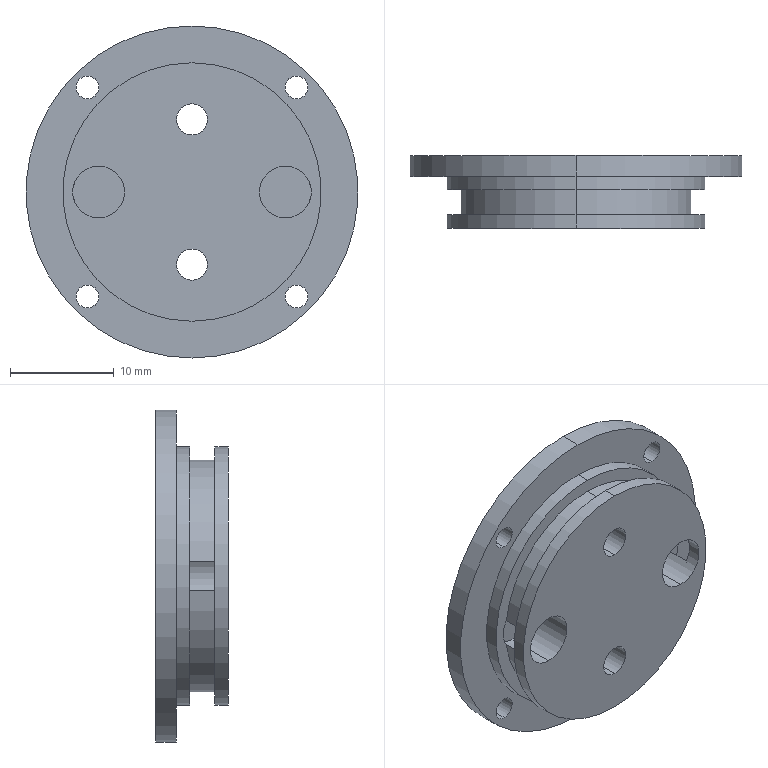Part | SolidWorks | features ICE 2, HoleWzd 1, Revolution 1 | 1 solid | 32 faces | box 32 x 7 x 32 mm | volume 3489 mm3 | cylinder 25 | plane 7 | commonest cylinder face diameters 2.2 x8 3 x4 5 x4 24.9 x4 22.309 x3 32 x2
STEP:
#1=CARTESIAN_POINT('',(0.,7.,-5.5));
#2=VERTEX_POINT('',#1);
#3=CARTESIAN_POINT('',(0.,7.,-8.5));
#4=VERTEX_POINT('',#3);
#5=CARTESIAN_POINT('',(0.,7.,-7.));
#6=DIRECTION('',(0.,-1.,0.));
#7=DIRECTION('',(0.,0.,-1.));
#8=AXIS2_PLACEMENT_3D('',#5,#6,#7);
#9=CIRCLE('',#8,1.5);
#10=EDGE_CURVE('',#2,#4,#9,.T.);
#11=ORIENTED_EDGE('',*,*,#10,.F.);
#12=CARTESIAN_POINT('',(0.,0.,-5.5));
#13=VERTEX_POINT('',#12);
#14=CARTESIAN_POINT('',(0.,5.,-5.5));
#15=DIRECTION('',(0.,-1.,0.));
#16=VECTOR('',#15,1000.);
#17=LINE('',#14,#16);
#18=EDGE_CURVE('',#2,#13,#17,.T.);
#19=ORIENTED_EDGE('',*,*,#18,.T.);
#20=CARTESIAN_POINT('',(0.,0.,-8.5));
#21=VERTEX_POINT('',#20);
#22=CARTESIAN_POINT('',(0.,0.,-7.));
#23=DIRECTION('',(0.,-1.,0.));
#24=DIRECTION('',(0.,0.,-1.));
#25=AXIS2_PLACEMENT_3D('',#22,#23,#24);
#26=CIRCLE('',#25,1.5);
#27=EDGE_CURVE('',#13,#21,#26,.T.);
#28=ORIENTED_EDGE('',*,*,#27,.T.);
#29=CARTESIAN_POINT('',(0.,5.,-8.5));
#30=DIRECTION('',(0.,-1.,0.));
#31=VECTOR('',#30,1000.);
#32=LINE('',#29,#31);
#33=EDGE_CURVE('',#4,#21,#32,.T.);
#34=ORIENTED_EDGE('',*,*,#33,.F.);
#35=EDGE_LOOP('',(#11,#19,#28,#34));
#36=FACE_OUTER_BOUND('',#35,.T.);
#37=CARTESIAN_POINT('',(0.,5.,-7.));
#38=DIRECTION('',(0.,-1.,0.));
#39=DIRECTION('',(0.,0.,-1.));
#40=AXIS2_PLACEMENT_3D('',#37,#38,#39);
#41=CYLINDRICAL_SURFACE('',#40,1.5);
#42=ADVANCED_FACE('',(#36),#41,.F.);
#43=CARTESIAN_POINT('',(0.,7.,8.5));
#44=VERTEX_POINT('',#43);
#45=CARTESIAN_POINT('',(0.,7.,5.5));
#46=VERTEX_POINT('',#45);
#47=CARTESIAN_POINT('',(0.,7.,7.));
#48=DIRECTION('',(0.,-1.,0.));
#49=DIRECTION('',(0.,0.,-1.));
#50=AXIS2_PLACEMENT_3D('',#47,#48,#49);
#51=CIRCLE('',#50,1.5);
#52=EDGE_CURVE('',#44,#46,#51,.T.);
#53=ORIENTED_EDGE('',*,*,#52,.F.);
#54=CARTESIAN_POINT('',(0.,0.,8.5));
#55=VERTEX_POINT('',#54);
#56=CARTESIAN_POINT('',(0.,5.,8.5));
#57=DIRECTION('',(0.,-1.,0.));
#58=VECTOR('',#57,1000.);
#59=LINE('',#56,#58);
#60=EDGE_CURVE('',#44,#55,#59,.T.);
#61=ORIENTED_EDGE('',*,*,#60,.T.);
#62=CARTESIAN_POINT('',(0.,0.,5.5));
#63=VERTEX_POINT('',#62);
#64=CARTESIAN_POINT('',(0.,0.,7.));
#65=DIRECTION('',(0.,-1.,0.));
#66=DIRECTION('',(0.,0.,-1.));
#67=AXIS2_PLACEMENT_3D('',#64,#65,#66);
#68=CIRCLE('',#67,1.5);
#69=EDGE_CURVE('',#55,#63,#68,.T.);
#70=ORIENTED_EDGE('',*,*,#69,.T.);
#71=CARTESIAN_POINT('',(0.,5.,5.5));
#72=DIRECTION('',(0.,-1.,0.));
#73=VECTOR('',#72,1000.);
#74=LINE('',#71,#73);
#75=EDGE_CURVE('',#46,#63,#74,.T.);
#76=ORIENTED_EDGE('',*,*,#75,.F.);
#77=EDGE_LOOP('',(#53,#61,#70,#76));
#78=FACE_OUTER_BOUND('',#77,.T.);
#79=CARTESIAN_POINT('',(0.,5.,7.));
#80=DIRECTION('',(0.,-1.,0.));
#81=DIRECTION('',(0.,0.,-1.));
#82=AXIS2_PLACEMENT_3D('',#79,#80,#81);
#83=CYLINDRICAL_SURFACE('',#82,1.5);
#84=ADVANCED_FACE('',(#78),#83,.F.);
#85=CARTESIAN_POINT('',(-11.065,3.708,1.409));
#86=VERTEX_POINT('',#85);
#87=CARTESIAN_POINT('',(-11.065,1.295,1.409));
#88=VERTEX_POINT('',#87);
#89=CARTESIAN_POINT('',(-11.065,2.5,1.409));
#90=DIRECTION('',(0.,-1.,0.));
#91=VECTOR('',#90,1000.);
#92=LINE('',#89,#91);
#93=EDGE_CURVE('',#86,#88,#92,.T.);
#94=ORIENTED_EDGE('',*,*,#93,.F.);
#95=CARTESIAN_POINT('',(-11.065,3.708,-1.409));
#96=VERTEX_POINT('',#95);
#97=CARTESIAN_POINT('',(-9.,3.708,0.));
#98=DIRECTION('',(0.,1.,0.));
#99=DIRECTION('',(0.,0.,1.));
#100=AXIS2_PLACEMENT_3D('',#97,#98,#99);
#101=CIRCLE('',#100,2.5);
#102=EDGE_CURVE('',#96,#86,#101,.T.);
#103=ORIENTED_EDGE('',*,*,#102,.F.);
#104=CARTESIAN_POINT('',(-11.065,1.295,-1.409));
#105=VERTEX_POINT('',#104);
#106=CARTESIAN_POINT('',(-11.065,2.5,-1.409));
#107=DIRECTION('',(0.,1.,0.));
#108=VECTOR('',#107,1000.);
#109=LINE('',#106,#108);
#110=EDGE_CURVE('',#105,#96,#109,.T.);
#111=ORIENTED_EDGE('',*,*,#110,.F.);
#112=CARTESIAN_POINT('',(-9.,1.295,0.));
#113=DIRECTION('',(0.,-1.,0.));
#114=DIRECTION('',(0.,0.,-1.));
#115=AXIS2_PLACEMENT_3D('',#112,#113,#114);
#116=CIRCLE('',#115,2.5);
#117=EDGE_CURVE('',#88,#105,#116,.T.);
#118=ORIENTED_EDGE('',*,*,#117,.F.);
#119=EDGE_LOOP('',(#94,#103,#111,#118));
#120=FACE_BOUND('',#119,.T.);
#121=CARTESIAN_POINT('',(-9.,5.,2.5));
#122=VERTEX_POINT('',#121);
#123=CARTESIAN_POINT('',(-9.,5.,-2.5));
#124=VERTEX_POINT('',#123);
#125=CARTESIAN_POINT('',(-9.,5.,0.));
#126=DIRECTION('',(0.,-1.,0.));
#127=DIRECTION('',(0.,0.,-1.));
#128=AXIS2_PLACEMENT_3D('',#125,#126,#127);
#129=CIRCLE('',#128,2.5);
#130=EDGE_CURVE('',#122,#124,#129,.T.);
#131=ORIENTED_EDGE('',*,*,#130,.F.);
#132=CARTESIAN_POINT('',(-9.,0.,2.5));
#133=VERTEX_POINT('',#132);
#134=CARTESIAN_POINT('',(-9.,5.,2.5));
#135=DIRECTION('',(0.,-1.,0.));
#136=VECTOR('',#135,1000.);
#137=LINE('',#134,#136);
#138=EDGE_CURVE('',#122,#133,#137,.T.);
#139=ORIENTED_EDGE('',*,*,#138,.T.);
#140=CARTESIAN_POINT('',(-9.,0.,-2.5));
#141=VERTEX_POINT('',#140);
#142=CARTESIAN_POINT('',(-9.,0.,0.));
#143=DIRECTION('',(0.,-1.,0.));
#144=DIRECTION('',(0.,0.,-1.));
#145=AXIS2_PLACEMENT_3D('',#142,#143,#144);
#146=CIRCLE('',#145,2.5);
#147=EDGE_CURVE('',#133,#141,#146,.T.);
#148=ORIENTED_EDGE('',*,*,#147,.T.);
#149=CARTESIAN_POINT('',(-9.,5.,-2.5));
#150=DIRECTION('',(0.,-1.,0.));
#151=VECTOR('',#150,1000.);
#152=LINE('',#149,#151);
#153=EDGE_CURVE('',#124,#141,#152,.T.);
#154=ORIENTED_EDGE('',*,*,#153,.F.);
#155=EDGE_LOOP('',(#131,#139,#148,#154));
#156=FACE_OUTER_BOUND('',#155,.T.);
#157=CARTESIAN_POINT('',(-9.,5.,0.));
#158=DIRECTION('',(0.,-1.,0.));
#159=DIRECTION('',(0.,0.,-1.));
#160=AXIS2_PLACEMENT_3D('',#157,#158,#159);
#161=CYLINDRICAL_SURFACE('',#160,2.5);
#162=ADVANCED_FACE('',(#120,#156),#161,.F.);
#163=CARTESIAN_POINT('',(9.,5.,2.5));
#164=VERTEX_POINT('',#163);
#165=CARTESIAN_POINT('',(9.,5.,-2.5));
#166=VERTEX_POINT('',#165);
#167=CARTESIAN_POINT('',(9.,5.,0.));
#168=DIRECTION('',(0.,-1.,0.));
#169=DIRECTION('',(0.,0.,-1.));
#170=AXIS2_PLACEMENT_3D('',#167,#168,#169);
#171=CIRCLE('',#170,2.5);
#172=EDGE_CURVE('',#164,#166,#171,.T.);
#173=ORIENTED_EDGE('',*,*,#172,.F.);
#174=CARTESIAN_POINT('',(9.,0.,2.5));
#175=VERTEX_POINT('',#174);
#176=CARTESIAN_POINT('',(9.,5.,2.5));
#177=DIRECTION('',(0.,-1.,0.));
#178=VECTOR('',#177,1000.);
#179=LINE('',#176,#178);
#180=EDGE_CURVE('',#164,#175,#179,.T.);
#181=ORIENTED_EDGE('',*,*,#180,.T.);
#182=CARTESIAN_POINT('',(9.,0.,-2.5));
#183=VERTEX_POINT('',#182);
#184=CARTESIAN_POINT('',(9.,0.,0.));
#185=DIRECTION('',(0.,-1.,0.));
#186=DIRECTION('',(0.,0.,-1.));
#187=AXIS2_PLACEMENT_3D('',#184,#185,#186);
#188=CIRCLE('',#187,2.5);
#189=EDGE_CURVE('',#175,#183,#188,.T.);
#190=ORIENTED_EDGE('',*,*,#189,.T.);
#191=CARTESIAN_POINT('',(9.,5.,-2.5));
#192=DIRECTION('',(0.,-1.,0.));
#193=VECTOR('',#192,1000.);
#194=LINE('',#191,#193);
#195=EDGE_CURVE('',#166,#183,#194,.T.);
#196=ORIENTED_EDGE('',*,*,#195,.F.);
#197=EDGE_LOOP('',(#173,#181,#190,#196));
#198=FACE_OUTER_BOUND('',#197,.T.);
#199=CARTESIAN_POINT('',(9.,5.,0.));
#200=DIRECTION('',(0.,-1.,0.));
#201=DIRECTION('',(0.,0.,-1.));
#202=AXIS2_PLACEMENT_3D('',#199,#200,#201);
#203=CYLINDRICAL_SURFACE('',#202,2.5);
#204=ADVANCED_FACE('',(#198),#203,.F.);
#205=CARTESIAN_POINT('',(-10.076,5.,-11.176));
#206=VERTEX_POINT('',#205);
#207=CARTESIAN_POINT('',(-10.076,5.,-8.976));
#208=VERTEX_POINT('',#207);
#209=CARTESIAN_POINT('',(-10.076,5.,-10.076));
#210=DIRECTION('',(0.,1.,0.));
#211=DIRECTION('',(0.,0.,1.));
#212=AXIS2_PLACEMENT_3D('',#209,#210,#211);
#213=CIRCLE('',#212,1.1);
#214=EDGE_CURVE('',#206,#208,#213,.T.);
#215=ORIENTED_EDGE('',*,*,#214,.F.);
#216=CARTESIAN_POINT('',(-10.076,7.,-11.176));
#217=VERTEX_POINT('',#216);
#218=CARTESIAN_POINT('',(-10.076,7.,-11.176));
#219=DIRECTION('',(0.,1.,0.));
#220=VECTOR('',#219,1000.);
#221=LINE('',#218,#220);
#222=EDGE_CURVE('',#206,#217,#221,.T.);
#223=ORIENTED_EDGE('',*,*,#222,.T.);
#224=CARTESIAN_POINT('',(-10.076,7.,-8.976));
#225=VERTEX_POINT('',#224);
#226=CARTESIAN_POINT('',(-10.076,7.,-10.076));
#227=DIRECTION('',(0.,1.,0.));
#228=DIRECTION('',(0.,0.,1.));
#229=AXIS2_PLACEMENT_3D('',#226,#227,#228);
#230=CIRCLE('',#229,1.1);
#231=EDGE_CURVE('',#217,#225,#230,.T.);
#232=ORIENTED_EDGE('',*,*,#231,.T.);
#233=CARTESIAN_POINT('',(-10.076,7.,-8.976));
#234=DIRECTION('',(0.,1.,0.));
#235=VECTOR('',#234,1000.);
#236=LINE('',#233,#235);
#237=EDGE_CURVE('',#208,#225,#236,.T.);
#238=ORIENTED_EDGE('',*,*,#237,.F.);
#239=EDGE_LOOP('',(#215,#223,#232,#238));
#240=FACE_OUTER_BOUND('',#239,.T.);
#241=CARTESIAN_POINT('',(-10.076,7.,-10.076));
#242=DIRECTION('',(0.,1.,0.));
#243=DIRECTION('',(0.,0.,1.));
#244=AXIS2_PLACEMENT_3D('',#241,#242,#243);
#245=CYLINDRICAL_SURFACE('',#244,1.1);
#246=ADVANCED_FACE('',(#240),#245,.F.);
#247=CARTESIAN_POINT('',(10.076,5.,-11.176));
#248=VERTEX_POINT('',#247);
#249=CARTESIAN_POINT('',(10.076,5.,-8.976));
#250=VERTEX_POINT('',#249);
#251=CARTESIAN_POINT('',(10.076,5.,-10.076));
#252=DIRECTION('',(0.,1.,0.));
#253=DIRECTION('',(0.,0.,1.));
#254=AXIS2_PLACEMENT_3D('',#251,#252,#253);
#255=CIRCLE('',#254,1.1);
#256=EDGE_CURVE('',#248,#250,#255,.T.);
#257=ORIENTED_EDGE('',*,*,#256,.F.);
#258=CARTESIAN_POINT('',(10.076,7.,-11.176));
#259=VERTEX_POINT('',#258);
#260=CARTESIAN_POINT('',(10.076,7.,-11.176));
#261=DIRECTION('',(0.,1.,0.));
#262=VECTOR('',#261,1000.);
#263=LINE('',#260,#262);
#264=EDGE_CURVE('',#248,#259,#263,.T.);
#265=ORIENTED_EDGE('',*,*,#264,.T.);
#266=CARTESIAN_POINT('',(10.076,7.,-8.976));
#267=VERTEX_POINT('',#266);
#268=CARTESIAN_POINT('',(10.076,7.,-10.076));
#269=DIRECTION('',(0.,1.,0.));
#270=DIRECTION('',(0.,0.,1.));
#271=AXIS2_PLACEMENT_3D('',#268,#269,#270);
#272=CIRCLE('',#271,1.1);
#273=EDGE_CURVE('',#259,#267,#272,.T.);
#274=ORIENTED_EDGE('',*,*,#273,.T.);
#275=CARTESIAN_POINT('',(10.076,7.,-8.976));
#276=DIRECTION('',(0.,1.,0.));
#277=VECTOR('',#276,1000.);
#278=LINE('',#275,#277);
#279=EDGE_CURVE('',#250,#267,#278,.T.);
#280=ORIENTED_EDGE('',*,*,#279,.F.);
#281=EDGE_LOOP('',(#257,#265,#274,#280));
#282=FACE_OUTER_BOUND('',#281,.T.);
#283=CARTESIAN_POINT('',(10.076,7.,-10.076));
#284=DIRECTION('',(0.,1.,0.));
#285=DIRECTION('',(0.,0.,1.));
#286=AXIS2_PLACEMENT_3D('',#283,#284,#285);
#287=CYLINDRICAL_SURFACE('',#286,1.1);
#288=ADVANCED_FACE('',(#282),#287,.F.);
#289=CARTESIAN_POINT('',(10.076,5.,8.976));
#290=VERTEX_POINT('',#289);
#291=CARTESIAN_POINT('',(10.076,5.,11.176));
#292=VERTEX_POINT('',#291);
#293=CARTESIAN_POINT('',(10.076,5.,10.076));
#294=DIRECTION('',(0.,1.,0.));
#295=DIRECTION('',(0.,0.,1.));
#296=AXIS2_PLACEMENT_3D('',#293,#294,#295);
#297=CIRCLE('',#296,1.1);
#298=EDGE_CURVE('',#290,#292,#297,.T.);
#299=ORIENTED_EDGE('',*,*,#298,.F.);
#300=CARTESIAN_POINT('',(10.076,7.,8.976));
#301=VERTEX_POINT('',#300);
#302=CARTESIAN_POINT('',(10.076,7.,8.976));
#303=DIRECTION('',(0.,1.,0.));
#304=VECTOR('',#303,1000.);
#305=LINE('',#302,#304);
#306=EDGE_CURVE('',#290,#301,#305,.T.);
#307=ORIENTED_EDGE('',*,*,#306,.T.);
#308=CARTESIAN_POINT('',(10.076,7.,11.176));
#309=VERTEX_POINT('',#308);
#310=CARTESIAN_POINT('',(10.076,7.,10.076));
#311=DIRECTION('',(0.,1.,0.));
#312=DIRECTION('',(0.,0.,1.));
#313=AXIS2_PLACEMENT_3D('',#310,#311,#312);
#314=CIRCLE('',#313,1.1);
#315=EDGE_CURVE('',#301,#309,#314,.T.);
#316=ORIENTED_EDGE('',*,*,#315,.T.);
#317=CARTESIAN_POINT('',(10.076,7.,11.176));
#318=DIRECTION('',(0.,1.,0.));
#319=VECTOR('',#318,1000.);
#320=LINE('',#317,#319);
#321=EDGE_CURVE('',#292,#309,#320,.T.);
#322=ORIENTED_EDGE('',*,*,#321,.F.);
#323=EDGE_LOOP('',(#299,#307,#316,#322));
#324=FACE_OUTER_BOUND('',#323,.T.);
#325=CARTESIAN_POINT('',(10.076,7.,10.076));
#326=DIRECTION('',(0.,1.,0.));
#327=DIRECTION('',(0.,0.,1.));
#328=AXIS2_PLACEMENT_3D('',#325,#326,#327);
#329=CYLINDRICAL_SURFACE('',#328,1.1);
#330=ADVANCED_FACE('',(#324),#329,.F.);
#331=CARTESIAN_POINT('',(-10.076,5.,8.976));
#332=VERTEX_POINT('',#331);
#333=CARTESIAN_POINT('',(-10.076,5.,11.176));
#334=VERTEX_POINT('',#333);
#335=CARTESIAN_POINT('',(-10.076,5.,10.076));
#336=DIRECTION('',(0.,1.,0.));
#337=DIRECTION('',(0.,0.,1.));
#338=AXIS2_PLACEMENT_3D('',#335,#336,#337);
#339=CIRCLE('',#338,1.1);
#340=EDGE_CURVE('',#332,#334,#339,.T.);
#341=ORIENTED_EDGE('',*,*,#340,.F.);
#342=CARTESIAN_POINT('',(-10.076,7.,8.976));
#343=VERTEX_POINT('',#342);
#344=CARTESIAN_POINT('',(-10.076,7.,8.976));
#345=DIRECTION('',(0.,1.,0.));
#346=VECTOR('',#345,1000.);
#347=LINE('',#344,#346);
#348=EDGE_CURVE('',#332,#343,#347,.T.);
#349=ORIENTED_EDGE('',*,*,#348,.T.);
#350=CARTESIAN_POINT('',(-10.076,7.,11.176));
#351=VERTEX_POINT('',#350);
#352=CARTESIAN_POINT('',(-10.076,7.,10.076));
#353=DIRECTION('',(0.,1.,0.));
#354=DIRECTION('',(0.,0.,1.));
#355=AXIS2_PLACEMENT_3D('',#352,#353,#354);
#356=CIRCLE('',#355,1.1);
#357=EDGE_CURVE('',#343,#351,#356,.T.);
#358=ORIENTED_EDGE('',*,*,#357,.T.);
#359=CARTESIAN_POINT('',(-10.076,7.,11.176));
#360=DIRECTION('',(0.,1.,0.));
#361=VECTOR('',#360,1000.);
#362=LINE('',#359,#361);
#363=EDGE_CURVE('',#334,#351,#362,.T.);
#364=ORIENTED_EDGE('',*,*,#363,.F.);
#365=EDGE_LOOP('',(#341,#349,#358,#364));
#366=FACE_OUTER_BOUND('',#365,.T.);
#367=CARTESIAN_POINT('',(-10.076,7.,10.076));
#368=DIRECTION('',(0.,1.,0.));
#369=DIRECTION('',(0.,0.,1.));
#370=AXIS2_PLACEMENT_3D('',#367,#368,#369);
#371=CYLINDRICAL_SURFACE('',#370,1.1);
#372=ADVANCED_FACE('',(#366),#371,.F.);
#373=CARTESIAN_POINT('',(0.,5.,16.));
#374=VERTEX_POINT('',#373);
#375=CARTESIAN_POINT('',(0.,5.,-16.));
#376=VERTEX_POINT('',#375);
#377=CARTESIAN_POINT('',(0.,5.,0.));
#378=DIRECTION('',(0.,1.,0.));
#379=DIRECTION('',(0.,0.,1.));
#380=AXIS2_PLACEMENT_3D('',#377,#378,#379);
#381=CIRCLE('',#380,16.);
#382=EDGE_CURVE('',#374,#376,#381,.T.);
#383=ORIENTED_EDGE('',*,*,#382,.T.);
#384=CARTESIAN_POINT('',(0.,7.,-16.));
#385=VERTEX_POINT('',#384);
#386=CARTESIAN_POINT('',(0.,7.,-16.));
#387=DIRECTION('',(0.,1.,0.));
#388=VECTOR('',#387,1000.);
#389=LINE('',#386,#388);
#390=EDGE_CURVE('',#376,#385,#389,.T.);
#391=ORIENTED_EDGE('',*,*,#390,.T.);
#392=CARTESIAN_POINT('',(0.,7.,16.));
#393=VERTEX_POINT('',#392);
#394=CARTESIAN_POINT('',(0.,7.,0.));
#395=DIRECTION('',(0.,1.,0.));
#396=DIRECTION('',(0.,0.,1.));
#397=AXIS2_PLACEMENT_3D('',#394,#395,#396);
#398=CIRCLE('',#397,16.);
#399=EDGE_CURVE('',#393,#385,#398,.T.);
#400=ORIENTED_EDGE('',*,*,#399,.F.);
#401=CARTESIAN_POINT('',(0.,7.,16.));
#402=DIRECTION('',(0.,1.,0.));
#403=VECTOR('',#402,1000.);
#404=LINE('',#401,#403);
#405=EDGE_CURVE('',#374,#393,#404,.T.);
#406=ORIENTED_EDGE('',*,*,#405,.F.);
#407=EDGE_LOOP('',(#383,#391,#400,#406));
#408=FACE_OUTER_BOUND('',#407,.T.);
#409=CARTESIAN_POINT('',(0.,7.,0.));
#410=DIRECTION('',(0.,1.,0.));
#411=DIRECTION('',(0.,0.,1.));
#412=AXIS2_PLACEMENT_3D('',#409,#410,#411);
#413=CYLINDRICAL_SURFACE('',#412,16.);
#414=ADVANCED_FACE('',(#408),#413,.T.);
#415=CARTESIAN_POINT('',(0.,3.708,12.45));
#416=VERTEX_POINT('',#415);
#417=CARTESIAN_POINT('',(0.,3.708,-12.45));
#418=VERTEX_POINT('',#417);
#419=CARTESIAN_POINT('',(0.,3.708,0.));
#420=DIRECTION('',(0.,1.,0.));
#421=DIRECTION('',(0.,0.,1.));
#422=AXIS2_PLACEMENT_3D('',#419,#420,#421);
#423=CIRCLE('',#422,12.45);
#424=EDGE_CURVE('',#416,#418,#423,.T.);
#425=ORIENTED_EDGE('',*,*,#424,.T.);
#426=CARTESIAN_POINT('',(0.,5.,-12.45));
#427=VERTEX_POINT('',#426);
#428=CARTESIAN_POINT('',(0.,7.,-12.45));
#429=DIRECTION('',(0.,1.,0.));
#430=VECTOR('',#429,1000.);
#431=LINE('',#428,#430);
#432=EDGE_CURVE('',#418,#427,#431,.T.);
#433=ORIENTED_EDGE('',*,*,#432,.T.);
#434=CARTESIAN_POINT('',(0.,5.,12.45));
#435=VERTEX_POINT('',#434);
#436=CARTESIAN_POINT('',(0.,5.,0.));
#437=DIRECTION('',(0.,1.,0.));
#438=DIRECTION('',(0.,0.,1.));
#439=AXIS2_PLACEMENT_3D('',#436,#437,#438);
#440=CIRCLE('',#439,12.45);
#441=EDGE_CURVE('',#435,#427,#440,.T.);
#442=ORIENTED_EDGE('',*,*,#441,.F.);
#443=CARTESIAN_POINT('',(0.,7.,12.45));
#444=DIRECTION('',(0.,1.,0.));
#445=VECTOR('',#444,1000.);
#446=LINE('',#443,#445);
#447=EDGE_CURVE('',#416,#435,#446,.T.);
#448=ORIENTED_EDGE('',*,*,#447,.F.);
#449=EDGE_LOOP('',(#425,#433,#442,#448));
#450=FACE_OUTER_BOUND('',#449,.T.);
#451=CARTESIAN_POINT('',(0.,7.,0.));
#452=DIRECTION('',(0.,1.,0.));
#453=DIRECTION('',(0.,0.,1.));
#454=AXIS2_PLACEMENT_3D('',#451,#452,#453);
#455=CYLINDRICAL_SURFACE('',#454,12.45);
#456=ADVANCED_FACE('',(#450),#455,.T.);
#457=CARTESIAN_POINT('',(0.,0.,12.45));
#458=VERTEX_POINT('',#457);
#459=CARTESIAN_POINT('',(0.,0.,-12.45));
#460=VERTEX_POINT('',#459);
#461=CARTESIAN_POINT('',(0.,0.,0.));
#462=DIRECTION('',(0.,1.,0.));
#463=DIRECTION('',(0.,0.,1.));
#464=AXIS2_PLACEMENT_3D('',#461,#462,#463);
#465=CIRCLE('',#464,12.45);
#466=EDGE_CURVE('',#458,#460,#465,.T.);
#467=ORIENTED_EDGE('',*,*,#466,.T.);
#468=CARTESIAN_POINT('',(0.,1.295,-12.45));
#469=VERTEX_POINT('',#468);
#470=CARTESIAN_POINT('',(0.,7.,-12.45));
#471=DIRECTION('',(0.,1.,0.));
#472=VECTOR('',#471,1000.);
#473=LINE('',#470,#472);
#474=EDGE_CURVE('',#460,#469,#473,.T.);
#475=ORIENTED_EDGE('',*,*,#474,.T.);
#476=CARTESIAN_POINT('',(0.,1.295,12.45));
#477=VERTEX_POINT('',#476);
#478=CARTESIAN_POINT('',(0.,1.295,0.));
#479=DIRECTION('',(0.,1.,0.));
#480=DIRECTION('',(0.,0.,1.));
#481=AXIS2_PLACEMENT_3D('',#478,#479,#480);
#482=CIRCLE('',#481,12.45);
#483=EDGE_CURVE('',#477,#469,#482,.T.);
#484=ORIENTED_EDGE('',*,*,#483,.F.);
#485=CARTESIAN_POINT('',(0.,7.,12.45));
#486=DIRECTION('',(0.,1.,0.));
#487=VECTOR('',#486,1000.);
#488=LINE('',#485,#487);
#489=EDGE_CURVE('',#458,#477,#488,.T.);
#490=ORIENTED_EDGE('',*,*,#489,.F.);
#491=EDGE_LOOP('',(#467,#475,#484,#490));
#492=FACE_OUTER_BOUND('',#491,.T.);
#493=CARTESIAN_POINT('',(0.,7.,0.));
#494=DIRECTION('',(0.,1.,0.));
#495=DIRECTION('',(0.,0.,1.));
#496=AXIS2_PLACEMENT_3D('',#493,#494,#495);
#497=CYLINDRICAL_SURFACE('',#496,12.45);
#498=ADVANCED_FACE('',(#492),#497,.T.);
#499=CARTESIAN_POINT('',(0.,1.295,11.155));
#500=VERTEX_POINT('',#499);
#501=CARTESIAN_POINT('',(0.,1.295,0.));
#502=DIRECTION('',(0.,1.,0.));
#503=DIRECTION('',(0.,0.,1.));
#504=AXIS2_PLACEMENT_3D('',#501,#502,#503);
#505=CIRCLE('',#504,11.155);
#506=EDGE_CURVE('',#88,#500,#505,.T.);
#507=ORIENTED_EDGE('',*,*,#506,.T.);
#508=CARTESIAN_POINT('',(0.,3.708,11.155));
#509=VERTEX_POINT('',#508);
#510=CARTESIAN_POINT('',(0.,7.,11.155));
#511=DIRECTION('',(0.,1.,0.));
#512=VECTOR('',#511,1000.);
#513=LINE('',#510,#512);
#514=EDGE_CURVE('',#500,#509,#513,.T.);
#515=ORIENTED_EDGE('',*,*,#514,.T.);
#516=CARTESIAN_POINT('',(0.,3.708,0.));
#517=DIRECTION('',(0.,1.,0.));
#518=DIRECTION('',(0.,0.,1.));
#519=AXIS2_PLACEMENT_3D('',#516,#517,#518);
#520=CIRCLE('',#519,11.155);
#521=EDGE_CURVE('',#86,#509,#520,.T.);
#522=ORIENTED_EDGE('',*,*,#521,.F.);
#523=ORIENTED_EDGE('',*,*,#93,.T.);
#524=EDGE_LOOP('',(#507,#515,#522,#523));
#525=FACE_OUTER_BOUND('',#524,.T.);
#526=CARTESIAN_POINT('',(0.,7.,0.));
#527=DIRECTION('',(0.,1.,0.));
#528=DIRECTION('',(0.,0.,1.));
#529=AXIS2_PLACEMENT_3D('',#526,#527,#528);
#530=CYLINDRICAL_SURFACE('',#529,11.155);
#531=ADVANCED_FACE('',(#525),#530,.T.);
#532=ORIENTED_EDGE('',*,*,#514,.F.);
#533=CARTESIAN_POINT('',(11.065,1.295,1.409));
#534=VERTEX_POINT('',#533);
#535=CARTESIAN_POINT('',(0.,1.295,0.));
#536=DIRECTION('',(0.,1.,0.));
#537=DIRECTION('',(0.,0.,1.));
#538=AXIS2_PLACEMENT_3D('',#535,#536,#537);
#539=CIRCLE('',#538,11.155);
#540=EDGE_CURVE('',#500,#534,#539,.T.);
#541=ORIENTED_EDGE('',*,*,#540,.T.);
#542=CARTESIAN_POINT('',(11.065,3.708,1.409));
#543=VERTEX_POINT('',#542);
#544=CARTESIAN_POINT('',(11.065,2.5,1.409));
#545=DIRECTION('',(0.,1.,0.));
#546=VECTOR('',#545,1000.);
#547=LINE('',#544,#546);
#548=EDGE_CURVE('',#534,#543,#547,.T.);
#549=ORIENTED_EDGE('',*,*,#548,.T.);
#550=CARTESIAN_POINT('',(0.,3.708,0.));
#551=DIRECTION('',(0.,1.,0.));
#552=DIRECTION('',(0.,0.,1.));
#553=AXIS2_PLACEMENT_3D('',#550,#551,#552);
#554=CIRCLE('',#553,11.155);
#555=EDGE_CURVE('',#509,#543,#554,.T.);
#556=ORIENTED_EDGE('',*,*,#555,.F.);
#557=EDGE_LOOP('',(#532,#541,#549,#556));
#558=FACE_OUTER_BOUND('',#557,.T.);
#559=CARTESIAN_POINT('',(0.,7.,0.));
#560=DIRECTION('',(0.,1.,0.));
#561=DIRECTION('',(0.,0.,1.));
#562=AXIS2_PLACEMENT_3D('',#559,#560,#561);
#563=CYLINDRICAL_SURFACE('',#562,11.155);
#564=ADVANCED_FACE('',(#558),#563,.T.);
#565=CARTESIAN_POINT('',(-9.,0.,0.));
#566=DIRECTION('',(0.,-1.,0.));
#567=DIRECTION('',(0.,0.,-1.));
#568=AXIS2_PLACEMENT_3D('',#565,#566,#567);
#569=CIRCLE('',#568,2.5);
#570=EDGE_CURVE('',#141,#133,#569,.T.);
#571=ORIENTED_EDGE('',*,*,#570,.F.);
#572=ORIENTED_EDGE('',*,*,#147,.F.);
#573=EDGE_LOOP('',(#571,#572));
#574=FACE_BOUND('',#573,.T.);
#575=CARTESIAN_POINT('',(9.,0.,0.));
#576=DIRECTION('',(0.,-1.,0.));
#577=DIRECTION('',(0.,0.,-1.));
#578=AXIS2_PLACEMENT_3D('',#575,#576,#577);
#579=CIRCLE('',#578,2.5);
#580=EDGE_CURVE('',#183,#175,#579,.T.);
#581=ORIENTED_EDGE('',*,*,#580,.F.);
#582=ORIENTED_EDGE('',*,*,#189,.F.);
#583=EDGE_LOOP('',(#581,#582));
#584=FACE_BOUND('',#583,.T.);
#585=CARTESIAN_POINT('',(0.,0.,-7.));
#586=DIRECTION('',(0.,-1.,0.));
#587=DIRECTION('',(0.,0.,-1.));
#588=AXIS2_PLACEMENT_3D('',#585,#586,#587);
#589=CIRCLE('',#588,1.5);
#590=EDGE_CURVE('',#21,#13,#589,.T.);
#591=ORIENTED_EDGE('',*,*,#590,.F.);
#592=ORIENTED_EDGE('',*,*,#27,.F.);
#593=EDGE_LOOP('',(#591,#592));
#594=FACE_BOUND('',#593,.T.);
#595=CARTESIAN_POINT('',(0.,0.,7.));
#596=DIRECTION('',(0.,-1.,0.));
#597=DIRECTION('',(0.,0.,-1.));
#598=AXIS2_PLACEMENT_3D('',#595,#596,#597);
#599=CIRCLE('',#598,1.5);
#600=EDGE_CURVE('',#63,#55,#599,.T.);
#601=ORIENTED_EDGE('',*,*,#600,.F.);
#602=ORIENTED_EDGE('',*,*,#69,.F.);
#603=EDGE_LOOP('',(#601,#602));
#604=FACE_BOUND('',#603,.T.);
#605=ORIENTED_EDGE('',*,*,#466,.F.);
#606=CARTESIAN_POINT('',(0.,0.,0.));
#607=DIRECTION('',(0.,1.,0.));
#608=DIRECTION('',(0.,0.,1.));
#609=AXIS2_PLACEMENT_3D('',#606,#607,#608);
#610=CIRCLE('',#609,12.45);
#611=EDGE_CURVE('',#460,#458,#610,.T.);
#612=ORIENTED_EDGE('',*,*,#611,.F.);
#613=EDGE_LOOP('',(#605,#612));
#614=FACE_OUTER_BOUND('',#613,.T.);
#615=CARTESIAN_POINT('',(0.,0.,0.));
#616=DIRECTION('',(0.,1.,0.));
#617=DIRECTION('',(0.,0.,1.));
#618=AXIS2_PLACEMENT_3D('',#615,#616,#617);
#619=PLANE('',#618);
#620=ADVANCED_FACE('',(#574,#584,#594,#604,#614),#619,.F.);
#621=ORIENTED_EDGE('',*,*,#474,.F.);
#622=ORIENTED_EDGE('',*,*,#611,.T.);
#623=ORIENTED_EDGE('',*,*,#489,.T.);
#624=CARTESIAN_POINT('',(0.,1.295,0.));
#625=DIRECTION('',(0.,1.,0.));
#626=DIRECTION('',(0.,0.,1.));
#627=AXIS2_PLACEMENT_3D('',#624,#625,#626);
#628=CIRCLE('',#627,12.45);
#629=EDGE_CURVE('',#469,#477,#628,.T.);
#630=ORIENTED_EDGE('',*,*,#629,.F.);
#631=EDGE_LOOP('',(#621,#622,#623,#630));
#632=FACE_OUTER_BOUND('',#631,.T.);
#633=CARTESIAN_POINT('',(0.,7.,0.));
#634=DIRECTION('',(0.,1.,0.));
#635=DIRECTION('',(0.,0.,1.));
#636=AXIS2_PLACEMENT_3D('',#633,#634,#635);
#637=CYLINDRICAL_SURFACE('',#636,12.45);
#638=ADVANCED_FACE('',(#632),#637,.T.);
#639=ORIENTED_EDGE('',*,*,#506,.F.);
#640=ORIENTED_EDGE('',*,*,#117,.T.);
#641=CARTESIAN_POINT('',(11.065,1.295,-1.409));
#642=VERTEX_POINT('',#641);
#643=CARTESIAN_POINT('',(0.,1.295,0.));
#644=DIRECTION('',(0.,1.,0.));
#645=DIRECTION('',(0.,0.,1.));
#646=AXIS2_PLACEMENT_3D('',#643,#644,#645);
#647=CIRCLE('',#646,11.155);
#648=EDGE_CURVE('',#642,#105,#647,.T.);
#649=ORIENTED_EDGE('',*,*,#648,.F.);
#650=CARTESIAN_POINT('',(9.,1.295,0.));
#651=DIRECTION('',(0.,-1.,0.));
#652=DIRECTION('',(0.,0.,-1.));
#653=AXIS2_PLACEMENT_3D('',#650,#651,#652);
#654=CIRCLE('',#653,2.5);
#655=EDGE_CURVE('',#642,#534,#654,.T.);
#656=ORIENTED_EDGE('',*,*,#655,.T.);
#657=ORIENTED_EDGE('',*,*,#540,.F.);
#658=EDGE_LOOP('',(#639,#640,#649,#656,#657));
#659=FACE_BOUND('',#658,.T.);
#660=ORIENTED_EDGE('',*,*,#483,.T.);
#661=ORIENTED_EDGE('',*,*,#629,.T.);
#662=EDGE_LOOP('',(#660,#661));
#663=FACE_OUTER_BOUND('',#662,.T.);
#664=CARTESIAN_POINT('',(12.45,1.295,0.));
#665=DIRECTION('',(0.,-1.,0.));
#666=DIRECTION('',(0.,0.,-1.));
#667=AXIS2_PLACEMENT_3D('',#664,#665,#666);
#668=PLANE('',#667);
#669=ADVANCED_FACE('',(#659,#663),#668,.F.);
#670=ORIENTED_EDGE('',*,*,#648,.T.);
#671=ORIENTED_EDGE('',*,*,#110,.T.);
#672=CARTESIAN_POINT('',(11.065,3.708,-1.409));
#673=VERTEX_POINT('',#672);
#674=CARTESIAN_POINT('',(0.,3.708,0.));
#675=DIRECTION('',(0.,1.,0.));
#676=DIRECTION('',(0.,0.,1.));
#677=AXIS2_PLACEMENT_3D('',#674,#675,#676);
#678=CIRCLE('',#677,11.155);
#679=EDGE_CURVE('',#673,#96,#678,.T.);
#680=ORIENTED_EDGE('',*,*,#679,.F.);
#681=CARTESIAN_POINT('',(11.065,2.5,-1.409));
#682=DIRECTION('',(0.,-1.,0.));
#683=VECTOR('',#682,1000.);
#684=LINE('',#681,#683);
#685=EDGE_CURVE('',#673,#642,#684,.T.);
#686=ORIENTED_EDGE('',*,*,#685,.T.);
#687=EDGE_LOOP('',(#670,#671,#680,#686));
#688=FACE_OUTER_BOUND('',#687,.T.);
#689=CARTESIAN_POINT('',(0.,7.,0.));
#690=DIRECTION('',(0.,1.,0.));
#691=DIRECTION('',(0.,0.,1.));
#692=AXIS2_PLACEMENT_3D('',#689,#690,#691);
#693=CYLINDRICAL_SURFACE('',#692,11.155);
#694=ADVANCED_FACE('',(#688),#693,.T.);
#695=ORIENTED_EDGE('',*,*,#424,.F.);
#696=CARTESIAN_POINT('',(0.,3.708,0.));
#697=DIRECTION('',(0.,1.,0.));
#698=DIRECTION('',(0.,0.,1.));
#699=AXIS2_PLACEMENT_3D('',#696,#697,#698);
#700=CIRCLE('',#699,12.45);
#701=EDGE_CURVE('',#418,#416,#700,.T.);
#702=ORIENTED_EDGE('',*,*,#701,.F.);
#703=EDGE_LOOP('',(#695,#702));
#704=FACE_OUTER_BOUND('',#703,.T.);
#705=ORIENTED_EDGE('',*,*,#679,.T.);
#706=ORIENTED_EDGE('',*,*,#102,.T.);
#707=ORIENTED_EDGE('',*,*,#521,.T.);
#708=ORIENTED_EDGE('',*,*,#555,.T.);
#709=CARTESIAN_POINT('',(9.,3.708,0.));
#710=DIRECTION('',(0.,1.,0.));
#711=DIRECTION('',(0.,0.,1.));
#712=AXIS2_PLACEMENT_3D('',#709,#710,#711);
#713=CIRCLE('',#712,2.5);
#714=EDGE_CURVE('',#543,#673,#713,.T.);
#715=ORIENTED_EDGE('',*,*,#714,.T.);
#716=EDGE_LOOP('',(#705,#706,#707,#708,#715));
#717=FACE_BOUND('',#716,.T.);
#718=CARTESIAN_POINT('',(11.155,3.708,0.));
#719=DIRECTION('',(0.,1.,0.));
#720=DIRECTION('',(0.,0.,1.));
#721=AXIS2_PLACEMENT_3D('',#718,#719,#720);
#722=PLANE('',#721);
#723=ADVANCED_FACE('',(#704,#717),#722,.F.);
#724=ORIENTED_EDGE('',*,*,#432,.F.);
#725=ORIENTED_EDGE('',*,*,#701,.T.);
#726=ORIENTED_EDGE('',*,*,#447,.T.);
#727=CARTESIAN_POINT('',(0.,5.,0.));
#728=DIRECTION('',(0.,1.,0.));
#729=DIRECTION('',(0.,0.,1.));
#730=AXIS2_PLACEMENT_3D('',#727,#728,#729);
#731=CIRCLE('',#730,12.45);
#732=EDGE_CURVE('',#427,#435,#731,.T.);
#733=ORIENTED_EDGE('',*,*,#732,.F.);
#734=EDGE_LOOP('',(#724,#725,#726,#733));
#735=FACE_OUTER_BOUND('',#734,.T.);
#736=CARTESIAN_POINT('',(0.,7.,0.));
#737=DIRECTION('',(0.,1.,0.));
#738=DIRECTION('',(0.,0.,1.));
#739=AXIS2_PLACEMENT_3D('',#736,#737,#738);
#740=CYLINDRICAL_SURFACE('',#739,12.45);
#741=ADVANCED_FACE('',(#735),#740,.T.);
#742=CARTESIAN_POINT('',(-10.076,5.,-10.076));
#743=DIRECTION('',(0.,1.,0.));
#744=DIRECTION('',(0.,0.,1.));
#745=AXIS2_PLACEMENT_3D('',#742,#743,#744);
#746=CIRCLE('',#745,1.1);
#747=EDGE_CURVE('',#208,#206,#746,.T.);
#748=ORIENTED_EDGE('',*,*,#747,.T.);
#749=ORIENTED_EDGE('',*,*,#214,.T.);
#750=EDGE_LOOP('',(#748,#749));
#751=FACE_BOUND('',#750,.T.);
#752=CARTESIAN_POINT('',(10.076,5.,-10.076));
#753=DIRECTION('',(0.,1.,0.));
#754=DIRECTION('',(0.,0.,1.));
#755=AXIS2_PLACEMENT_3D('',#752,#753,#754);
#756=CIRCLE('',#755,1.1);
#757=EDGE_CURVE('',#250,#248,#756,.T.);
#758=ORIENTED_EDGE('',*,*,#757,.T.);
#759=ORIENTED_EDGE('',*,*,#256,.T.);
#760=EDGE_LOOP('',(#758,#759));
#761=FACE_BOUND('',#760,.T.);
#762=CARTESIAN_POINT('',(10.076,5.,10.076));
#763=DIRECTION('',(0.,1.,0.));
#764=DIRECTION('',(0.,0.,1.));
#765=AXIS2_PLACEMENT_3D('',#762,#763,#764);
#766=CIRCLE('',#765,1.1);
#767=EDGE_CURVE('',#292,#290,#766,.T.);
#768=ORIENTED_EDGE('',*,*,#767,.T.);
#769=ORIENTED_EDGE('',*,*,#298,.T.);
#770=EDGE_LOOP('',(#768,#769));
#771=FACE_BOUND('',#770,.T.);
#772=CARTESIAN_POINT('',(-10.076,5.,10.076));
#773=DIRECTION('',(0.,1.,0.));
#774=DIRECTION('',(0.,0.,1.));
#775=AXIS2_PLACEMENT_3D('',#772,#773,#774);
#776=CIRCLE('',#775,1.1);
#777=EDGE_CURVE('',#334,#332,#776,.T.);
#778=ORIENTED_EDGE('',*,*,#777,.T.);
#779=ORIENTED_EDGE('',*,*,#340,.T.);
#780=EDGE_LOOP('',(#778,#779));
#781=FACE_BOUND('',#780,.T.);
#782=ORIENTED_EDGE('',*,*,#382,.F.);
#783=CARTESIAN_POINT('',(0.,5.,0.));
#784=DIRECTION('',(0.,1.,0.));
#785=DIRECTION('',(0.,0.,1.));
#786=AXIS2_PLACEMENT_3D('',#783,#784,#785);
#787=CIRCLE('',#786,16.);
#788=EDGE_CURVE('',#376,#374,#787,.T.);
#789=ORIENTED_EDGE('',*,*,#788,.F.);
#790=EDGE_LOOP('',(#782,#789));
#791=FACE_OUTER_BOUND('',#790,.T.);
#792=ORIENTED_EDGE('',*,*,#441,.T.);
#793=ORIENTED_EDGE('',*,*,#732,.T.);
#794=EDGE_LOOP('',(#792,#793));
#795=FACE_BOUND('',#794,.T.);
#796=CARTESIAN_POINT('',(12.45,5.,0.));
#797=DIRECTION('',(0.,1.,0.));
#798=DIRECTION('',(0.,0.,1.));
#799=AXIS2_PLACEMENT_3D('',#796,#797,#798);
#800=PLANE('',#799);
#801=ADVANCED_FACE('',(#751,#761,#771,#781,#791,#795),#800,.F.);
#802=ORIENTED_EDGE('',*,*,#390,.F.);
#803=ORIENTED_EDGE('',*,*,#788,.T.);
#804=ORIENTED_EDGE('',*,*,#405,.T.);
#805=CARTESIAN_POINT('',(0.,7.,0.));
#806=DIRECTION('',(0.,1.,0.));
#807=DIRECTION('',(0.,0.,1.));
#808=AXIS2_PLACEMENT_3D('',#805,#806,#807);
#809=CIRCLE('',#808,16.);
#810=EDGE_CURVE('',#385,#393,#809,.T.);
#811=ORIENTED_EDGE('',*,*,#810,.F.);
#812=EDGE_LOOP('',(#802,#803,#804,#811));
#813=FACE_OUTER_BOUND('',#812,.T.);
#814=CARTESIAN_POINT('',(0.,7.,0.));
#815=DIRECTION('',(0.,1.,0.));
#816=DIRECTION('',(0.,0.,1.));
#817=AXIS2_PLACEMENT_3D('',#814,#815,#816);
#818=CYLINDRICAL_SURFACE('',#817,16.);
#819=ADVANCED_FACE('',(#813),#818,.T.);
#820=CARTESIAN_POINT('',(0.,7.,7.));
#821=DIRECTION('',(0.,-1.,0.));
#822=DIRECTION('',(0.,0.,-1.));
#823=AXIS2_PLACEMENT_3D('',#820,#821,#822);
#824=CIRCLE('',#823,1.5);
#825=EDGE_CURVE('',#46,#44,#824,.T.);
#826=ORIENTED_EDGE('',*,*,#825,.T.);
#827=ORIENTED_EDGE('',*,*,#52,.T.);
#828=EDGE_LOOP('',(#826,#827));
#829=FACE_BOUND('',#828,.T.);
#830=CARTESIAN_POINT('',(0.,7.,-7.));
#831=DIRECTION('',(0.,-1.,0.));
#832=DIRECTION('',(0.,0.,-1.));
#833=AXIS2_PLACEMENT_3D('',#830,#831,#832);
#834=CIRCLE('',#833,1.5);
#835=EDGE_CURVE('',#4,#2,#834,.T.);
#836=ORIENTED_EDGE('',*,*,#835,.T.);
#837=ORIENTED_EDGE('',*,*,#10,.T.);
#838=EDGE_LOOP('',(#836,#837));
#839=FACE_BOUND('',#838,.T.);
#840=CARTESIAN_POINT('',(-10.076,7.,-10.076));
#841=DIRECTION('',(0.,1.,0.));
#842=DIRECTION('',(0.,0.,1.));
#843=AXIS2_PLACEMENT_3D('',#840,#841,#842);
#844=CIRCLE('',#843,1.1);
#845=EDGE_CURVE('',#225,#217,#844,.T.);
#846=ORIENTED_EDGE('',*,*,#845,.F.);
#847=ORIENTED_EDGE('',*,*,#231,.F.);
#848=EDGE_LOOP('',(#846,#847));
#849=FACE_BOUND('',#848,.T.);
#850=CARTESIAN_POINT('',(10.076,7.,-10.076));
#851=DIRECTION('',(0.,1.,0.));
#852=DIRECTION('',(0.,0.,1.));
#853=AXIS2_PLACEMENT_3D('',#850,#851,#852);
#854=CIRCLE('',#853,1.1);
#855=EDGE_CURVE('',#267,#259,#854,.T.);
#856=ORIENTED_EDGE('',*,*,#855,.F.);
#857=ORIENTED_EDGE('',*,*,#273,.F.);
#858=EDGE_LOOP('',(#856,#857));
#859=FACE_BOUND('',#858,.T.);
#860=CARTESIAN_POINT('',(10.076,7.,10.076));
#861=DIRECTION('',(0.,1.,0.));
#862=DIRECTION('',(0.,0.,1.));
#863=AXIS2_PLACEMENT_3D('',#860,#861,#862);
#864=CIRCLE('',#863,1.1);
#865=EDGE_CURVE('',#309,#301,#864,.T.);
#866=ORIENTED_EDGE('',*,*,#865,.F.);
#867=ORIENTED_EDGE('',*,*,#315,.F.);
#868=EDGE_LOOP('',(#866,#867));
#869=FACE_BOUND('',#868,.T.);
#870=CARTESIAN_POINT('',(-10.076,7.,10.076));
#871=DIRECTION('',(0.,1.,0.));
#872=DIRECTION('',(0.,0.,1.));
#873=AXIS2_PLACEMENT_3D('',#870,#871,#872);
#874=CIRCLE('',#873,1.1);
#875=EDGE_CURVE('',#351,#343,#874,.T.);
#876=ORIENTED_EDGE('',*,*,#875,.F.);
#877=ORIENTED_EDGE('',*,*,#357,.F.);
#878=EDGE_LOOP('',(#876,#877));
#879=FACE_BOUND('',#878,.T.);
#880=ORIENTED_EDGE('',*,*,#399,.T.);
#881=ORIENTED_EDGE('',*,*,#810,.T.);
#882=EDGE_LOOP('',(#880,#881));
#883=FACE_OUTER_BOUND('',#882,.T.);
#884=CARTESIAN_POINT('',(16.,7.,0.));
#885=DIRECTION('',(0.,-1.,0.));
#886=DIRECTION('',(0.,0.,-1.));
#887=AXIS2_PLACEMENT_3D('',#884,#885,#886);
#888=PLANE('',#887);
#889=ADVANCED_FACE('',(#829,#839,#849,#859,#869,#879,#883),#888,.F.);
#890=ORIENTED_EDGE('',*,*,#348,.F.);
#891=ORIENTED_EDGE('',*,*,#777,.F.);
#892=ORIENTED_EDGE('',*,*,#363,.T.);
#893=ORIENTED_EDGE('',*,*,#875,.T.);
#894=EDGE_LOOP('',(#890,#891,#892,#893));
#895=FACE_OUTER_BOUND('',#894,.T.);
#896=CARTESIAN_POINT('',(-10.076,7.,10.076));
#897=DIRECTION('',(0.,1.,0.));
#898=DIRECTION('',(0.,0.,1.));
#899=AXIS2_PLACEMENT_3D('',#896,#897,#898);
#900=CYLINDRICAL_SURFACE('',#899,1.1);
#901=ADVANCED_FACE('',(#895),#900,.F.);
#902=ORIENTED_EDGE('',*,*,#306,.F.);
#903=ORIENTED_EDGE('',*,*,#767,.F.);
#904=ORIENTED_EDGE('',*,*,#321,.T.);
#905=ORIENTED_EDGE('',*,*,#865,.T.);
#906=EDGE_LOOP('',(#902,#903,#904,#905));
#907=FACE_OUTER_BOUND('',#906,.T.);
#908=CARTESIAN_POINT('',(10.076,7.,10.076));
#909=DIRECTION('',(0.,1.,0.));
#910=DIRECTION('',(0.,0.,1.));
#911=AXIS2_PLACEMENT_3D('',#908,#909,#910);
#912=CYLINDRICAL_SURFACE('',#911,1.1);
#913=ADVANCED_FACE('',(#907),#912,.F.);
#914=ORIENTED_EDGE('',*,*,#264,.F.);
#915=ORIENTED_EDGE('',*,*,#757,.F.);
#916=ORIENTED_EDGE('',*,*,#279,.T.);
#917=ORIENTED_EDGE('',*,*,#855,.T.);
#918=EDGE_LOOP('',(#914,#915,#916,#917));
#919=FACE_OUTER_BOUND('',#918,.T.);
#920=CARTESIAN_POINT('',(10.076,7.,-10.076));
#921=DIRECTION('',(0.,1.,0.));
#922=DIRECTION('',(0.,0.,1.));
#923=AXIS2_PLACEMENT_3D('',#920,#921,#922);
#924=CYLINDRICAL_SURFACE('',#923,1.1);
#925=ADVANCED_FACE('',(#919),#924,.F.);
#926=ORIENTED_EDGE('',*,*,#222,.F.);
#927=ORIENTED_EDGE('',*,*,#747,.F.);
#928=ORIENTED_EDGE('',*,*,#237,.T.);
#929=ORIENTED_EDGE('',*,*,#845,.T.);
#930=EDGE_LOOP('',(#926,#927,#928,#929));
#931=FACE_OUTER_BOUND('',#930,.T.);
#932=CARTESIAN_POINT('',(-10.076,7.,-10.076));
#933=DIRECTION('',(0.,1.,0.));
#934=DIRECTION('',(0.,0.,1.));
#935=AXIS2_PLACEMENT_3D('',#932,#933,#934);
#936=CYLINDRICAL_SURFACE('',#935,1.1);
#937=ADVANCED_FACE('',(#931),#936,.F.);
#938=ORIENTED_EDGE('',*,*,#180,.F.);
#939=CARTESIAN_POINT('',(9.,5.,0.));
#940=DIRECTION('',(0.,-1.,0.));
#941=DIRECTION('',(0.,0.,-1.));
#942=AXIS2_PLACEMENT_3D('',#939,#940,#941);
#943=CIRCLE('',#942,2.5);
#944=EDGE_CURVE('',#166,#164,#943,.T.);
#945=ORIENTED_EDGE('',*,*,#944,.F.);
#946=ORIENTED_EDGE('',*,*,#195,.T.);
#947=ORIENTED_EDGE('',*,*,#580,.T.);
#948=EDGE_LOOP('',(#938,#945,#946,#947));
#949=FACE_OUTER_BOUND('',#948,.T.);
#950=ORIENTED_EDGE('',*,*,#685,.F.);
#951=ORIENTED_EDGE('',*,*,#714,.F.);
#952=ORIENTED_EDGE('',*,*,#548,.F.);
#953=ORIENTED_EDGE('',*,*,#655,.F.);
#954=EDGE_LOOP('',(#950,#951,#952,#953));
#955=FACE_BOUND('',#954,.T.);
#956=CARTESIAN_POINT('',(9.,5.,0.));
#957=DIRECTION('',(0.,-1.,0.));
#958=DIRECTION('',(0.,0.,-1.));
#959=AXIS2_PLACEMENT_3D('',#956,#957,#958);
#960=CYLINDRICAL_SURFACE('',#959,2.5);
#961=ADVANCED_FACE('',(#949,#955),#960,.F.);
#962=ORIENTED_EDGE('',*,*,#944,.T.);
#963=ORIENTED_EDGE('',*,*,#172,.T.);
#964=EDGE_LOOP('',(#962,#963));
#965=FACE_OUTER_BOUND('',#964,.T.);
#966=CARTESIAN_POINT('',(9.,5.,0.));
#967=DIRECTION('',(0.,-1.,0.));
#968=DIRECTION('',(0.,0.,-1.));
#969=AXIS2_PLACEMENT_3D('',#966,#967,#968);
#970=PLANE('',#969);
#971=ADVANCED_FACE('',(#965),#970,.T.);
#972=ORIENTED_EDGE('',*,*,#138,.F.);
#973=CARTESIAN_POINT('',(-9.,5.,0.));
#974=DIRECTION('',(0.,-1.,0.));
#975=DIRECTION('',(0.,0.,-1.));
#976=AXIS2_PLACEMENT_3D('',#973,#974,#975);
#977=CIRCLE('',#976,2.5);
#978=EDGE_CURVE('',#124,#122,#977,.T.);
#979=ORIENTED_EDGE('',*,*,#978,.F.);
#980=ORIENTED_EDGE('',*,*,#153,.T.);
#981=ORIENTED_EDGE('',*,*,#570,.T.);
#982=EDGE_LOOP('',(#972,#979,#980,#981));
#983=FACE_OUTER_BOUND('',#982,.T.);
#984=CARTESIAN_POINT('',(-9.,5.,0.));
#985=DIRECTION('',(0.,-1.,0.));
#986=DIRECTION('',(0.,0.,-1.));
#987=AXIS2_PLACEMENT_3D('',#984,#985,#986);
#988=CYLINDRICAL_SURFACE('',#987,2.5);
#989=ADVANCED_FACE('',(#983),#988,.F.);
#990=ORIENTED_EDGE('',*,*,#978,.T.);
#991=ORIENTED_EDGE('',*,*,#130,.T.);
#992=EDGE_LOOP('',(#990,#991));
#993=FACE_OUTER_BOUND('',#992,.T.);
#994=CARTESIAN_POINT('',(-9.,5.,0.));
#995=DIRECTION('',(0.,-1.,0.));
#996=DIRECTION('',(0.,0.,-1.));
#997=AXIS2_PLACEMENT_3D('',#994,#995,#996);
#998=PLANE('',#997);
#999=ADVANCED_FACE('',(#993),#998,.T.);
#1000=ORIENTED_EDGE('',*,*,#60,.F.);
#1001=ORIENTED_EDGE('',*,*,#825,.F.);
#1002=ORIENTED_EDGE('',*,*,#75,.T.);
#1003=ORIENTED_EDGE('',*,*,#600,.T.);
#1004=EDGE_LOOP('',(#1000,#1001,#1002,#1003));
#1005=FACE_OUTER_BOUND('',#1004,.T.);
#1006=CARTESIAN_POINT('',(0.,5.,7.));
#1007=DIRECTION('',(0.,-1.,0.));
#1008=DIRECTION('',(0.,0.,-1.));
#1009=AXIS2_PLACEMENT_3D('',#1006,#1007,#1008);
#1010=CYLINDRICAL_SURFACE('',#1009,1.5);
#1011=ADVANCED_FACE('',(#1005),#1010,.F.);
#1012=ORIENTED_EDGE('',*,*,#18,.F.);
#1013=ORIENTED_EDGE('',*,*,#835,.F.);
#1014=ORIENTED_EDGE('',*,*,#33,.T.);
#1015=ORIENTED_EDGE('',*,*,#590,.T.);
#1016=EDGE_LOOP('',(#1012,#1013,#1014,#1015));
#1017=FACE_OUTER_BOUND('',#1016,.T.);
#1018=CARTESIAN_POINT('',(0.,5.,-7.));
#1019=DIRECTION('',(0.,-1.,0.));
#1020=DIRECTION('',(0.,0.,-1.));
#1021=AXIS2_PLACEMENT_3D('',#1018,#1019,#1020);
#1022=CYLINDRICAL_SURFACE('',#1021,1.5);
#1023=ADVANCED_FACE('',(#1017),#1022,.F.);
#1024=CLOSED_SHELL('',(#42,#84,#162,#204,#246,#288,#330,#372,#414,#456,#498,#531,#564,#620,#638,#669,#694,#723,#741,#801,#819,#889,#901,#913,#925,#937,#961,#971,#989,#999,#1011,#1023));
#1025=MANIFOLD_SOLID_BREP('',#1024);
#1026=CARTESIAN_POINT('',(0.,0.,0.));
#1027=DIRECTION('',(0.,0.,1.));
#1028=DIRECTION('',(1.,0.,0.));
#1029=AXIS2_PLACEMENT_3D('',#1026,#1027,#1028);
#1030=(LENGTH_UNIT()NAMED_UNIT(*)SI_UNIT(.MILLI.,.METRE.));
#1031=UNCERTAINTY_MEASURE_WITH_UNIT(LENGTH_MEASURE(0.00001),#1030,'','');
#1032=(NAMED_UNIT(*)PLANE_ANGLE_UNIT()SI_UNIT($,.RADIAN.));
#1033=(NAMED_UNIT(*)SI_UNIT($,.STERADIAN.)SOLID_ANGLE_UNIT());
#1034=(GEOMETRIC_REPRESENTATION_CONTEXT(3)GLOBAL_UNCERTAINTY_ASSIGNED_CONTEXT((#1031))GLOBAL_UNIT_ASSIGNED_CONTEXT((#1030,#1032,#1033))REPRESENTATION_CONTEXT('',''));
#1035=ADVANCED_BREP_SHAPE_REPRESENTATION('',(#1025,#1029),#1034);